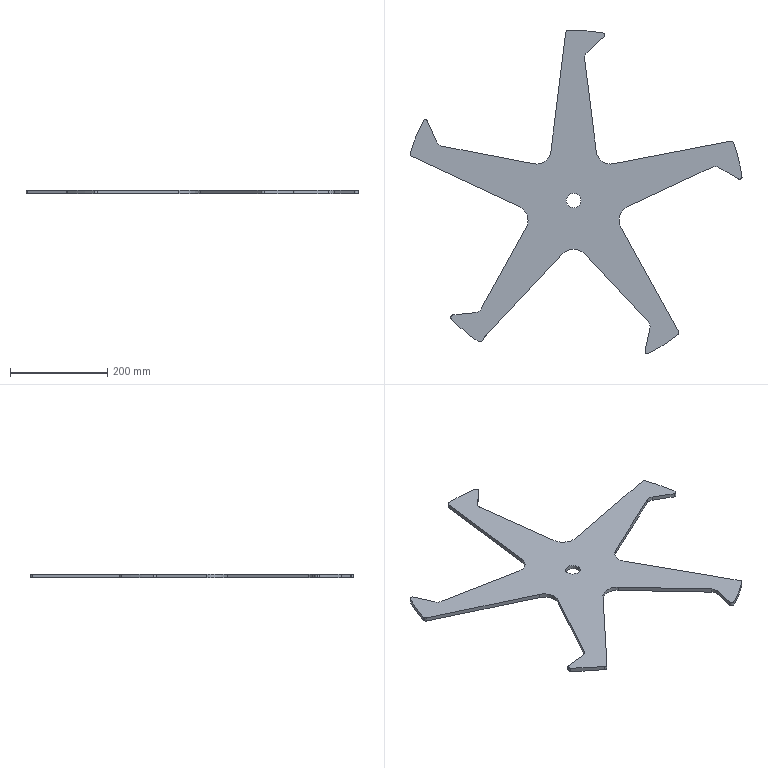Part | SolidWorks | features Extrusion 1 | 1 solid | 49 faces | box 682.923 x 664.717 x 8 mm | volume 939255 mm3 | cylinder 32 | plane 17 | commonest cylinder face diameters 10 x13 30 x8 60.749 x6 700 x5